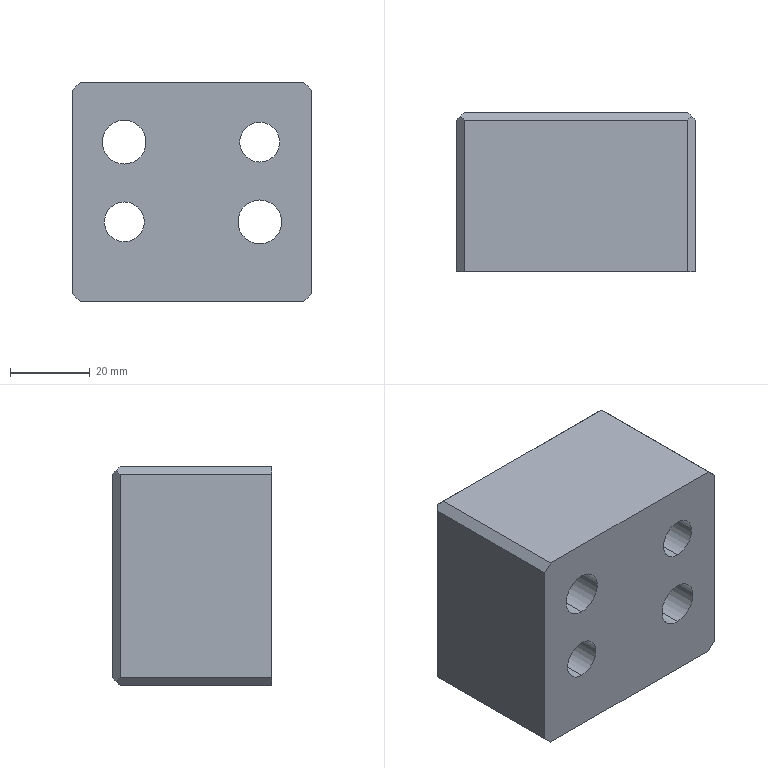Part | Creo | 1 solid | 28 faces | box 60 x 40 x 55 mm | volume 114572 mm3 | plane 16 | cylinder 12 | commonest cylinder face diameters 10 x4 11 x4 16.8 x4
STEP:
#1=CARTESIAN_POINT('',(-185.,390.,-37.));
#2=VERTEX_POINT('',#1);
#3=CARTESIAN_POINT('',(-241.,390.,-37.));
#4=VERTEX_POINT('',#3);
#5=CARTESIAN_POINT('',(-185.,390.,-37.));
#6=DIRECTION('',(-1.,0.,0.));
#7=VECTOR('',#6,56.);
#8=LINE('',#5,#7);
#9=EDGE_CURVE('',#2,#4,#8,.T.);
#10=ORIENTED_EDGE('',*,*,#9,.T.);
#11=CARTESIAN_POINT('',(-241.,390.,-88.));
#12=VERTEX_POINT('',#11);
#13=CARTESIAN_POINT('',(-241.,390.,-37.));
#14=DIRECTION('',(0.,0.,-1.));
#15=VECTOR('',#14,51.);
#16=LINE('',#13,#15);
#17=EDGE_CURVE('',#4,#12,#16,.T.);
#18=ORIENTED_EDGE('',*,*,#17,.T.);
#19=CARTESIAN_POINT('',(-185.,390.,-88.));
#20=VERTEX_POINT('',#19);
#21=CARTESIAN_POINT('',(-241.,390.,-88.));
#22=DIRECTION('',(1.,0.,0.));
#23=VECTOR('',#22,56.);
#24=LINE('',#21,#23);
#25=EDGE_CURVE('',#12,#20,#24,.T.);
#26=ORIENTED_EDGE('',*,*,#25,.T.);
#27=CARTESIAN_POINT('',(-185.,390.,-88.));
#28=DIRECTION('',(0.,0.,1.));
#29=VECTOR('',#28,51.);
#30=LINE('',#27,#29);
#31=EDGE_CURVE('',#20,#2,#30,.T.);
#32=ORIENTED_EDGE('',*,*,#31,.T.);
#33=EDGE_LOOP('',(#10,#18,#26,#32));
#34=FACE_OUTER_BOUND('',#33,.F.);
#35=CARTESIAN_POINT('',(-204.4,390.,-70.));
#36=VERTEX_POINT('',#35);
#37=CARTESIAN_POINT('',(-196.,390.,-78.4));
#38=VERTEX_POINT('',#37);
#39=CARTESIAN_POINT('',(-196.,390.,-70.));
#40=DIRECTION('',(0.,-1.,0.));
#41=DIRECTION('',(-1.,0.,0.));
#42=AXIS2_PLACEMENT_3D('',#39,#40,#41);
#43=CIRCLE('',#42,8.4);
#44=EDGE_CURVE('',#36,#38,#43,.T.);
#45=ORIENTED_EDGE('',*,*,#44,.F.);
#46=CARTESIAN_POINT('',(-196.,390.,-61.6));
#47=VERTEX_POINT('',#46);
#48=CARTESIAN_POINT('',(-196.,390.,-70.));
#49=DIRECTION('',(0.,-1.,0.));
#50=DIRECTION('',(0.,0.,1.));
#51=AXIS2_PLACEMENT_3D('',#48,#49,#50);
#52=CIRCLE('',#51,8.4);
#53=EDGE_CURVE('',#47,#36,#52,.T.);
#54=ORIENTED_EDGE('',*,*,#53,.F.);
#55=CARTESIAN_POINT('',(-196.,390.,-70.));
#56=DIRECTION('',(0.,-1.,0.));
#57=DIRECTION('',(0.,0.,-1.));
#58=AXIS2_PLACEMENT_3D('',#55,#56,#57);
#59=CIRCLE('',#58,8.4);
#60=EDGE_CURVE('',#38,#47,#59,.T.);
#61=ORIENTED_EDGE('',*,*,#60,.F.);
#62=EDGE_LOOP('',(#45,#54,#61));
#63=FACE_BOUND('',#62,.F.);
#64=CARTESIAN_POINT('',(-238.4,390.,-50.));
#65=VERTEX_POINT('',#64);
#66=CARTESIAN_POINT('',(-230.,390.,-58.4));
#67=VERTEX_POINT('',#66);
#68=CARTESIAN_POINT('',(-230.,390.,-50.));
#69=DIRECTION('',(0.,-1.,0.));
#70=DIRECTION('',(-1.,0.,0.));
#71=AXIS2_PLACEMENT_3D('',#68,#69,#70);
#72=CIRCLE('',#71,8.4);
#73=EDGE_CURVE('',#65,#67,#72,.T.);
#74=ORIENTED_EDGE('',*,*,#73,.F.);
#75=CARTESIAN_POINT('',(-230.,390.,-41.6));
#76=VERTEX_POINT('',#75);
#77=CARTESIAN_POINT('',(-230.,390.,-50.));
#78=DIRECTION('',(0.,-1.,0.));
#79=DIRECTION('',(0.,0.,1.));
#80=AXIS2_PLACEMENT_3D('',#77,#78,#79);
#81=CIRCLE('',#80,8.4);
#82=EDGE_CURVE('',#76,#65,#81,.T.);
#83=ORIENTED_EDGE('',*,*,#82,.F.);
#84=CARTESIAN_POINT('',(-230.,390.,-50.));
#85=DIRECTION('',(0.,-1.,0.));
#86=DIRECTION('',(0.,0.,-1.));
#87=AXIS2_PLACEMENT_3D('',#84,#85,#86);
#88=CIRCLE('',#87,8.4);
#89=EDGE_CURVE('',#67,#76,#88,.T.);
#90=ORIENTED_EDGE('',*,*,#89,.F.);
#91=EDGE_LOOP('',(#74,#83,#90));
#92=FACE_BOUND('',#91,.F.);
#93=CARTESIAN_POINT('',(-230.,390.,-75.));
#94=VERTEX_POINT('',#93);
#95=CARTESIAN_POINT('',(-230.,390.,-65.));
#96=VERTEX_POINT('',#95);
#97=CARTESIAN_POINT('',(-230.,390.,-70.));
#98=DIRECTION('',(0.,-1.,0.));
#99=DIRECTION('',(0.,0.,-1.));
#100=AXIS2_PLACEMENT_3D('',#97,#98,#99);
#101=CIRCLE('',#100,5.);
#102=EDGE_CURVE('',#94,#96,#101,.T.);
#103=ORIENTED_EDGE('',*,*,#102,.F.);
#104=CARTESIAN_POINT('',(-230.,390.,-70.));
#105=DIRECTION('',(0.,-1.,0.));
#106=DIRECTION('',(0.,0.,1.));
#107=AXIS2_PLACEMENT_3D('',#104,#105,#106);
#108=CIRCLE('',#107,5.);
#109=EDGE_CURVE('',#96,#94,#108,.T.);
#110=ORIENTED_EDGE('',*,*,#109,.F.);
#111=EDGE_LOOP('',(#103,#110));
#112=FACE_BOUND('',#111,.F.);
#113=CARTESIAN_POINT('',(-196.,390.,-55.));
#114=VERTEX_POINT('',#113);
#115=CARTESIAN_POINT('',(-196.,390.,-45.));
#116=VERTEX_POINT('',#115);
#117=CARTESIAN_POINT('',(-196.,390.,-50.));
#118=DIRECTION('',(0.,-1.,0.));
#119=DIRECTION('',(0.,0.,-1.));
#120=AXIS2_PLACEMENT_3D('',#117,#118,#119);
#121=CIRCLE('',#120,5.);
#122=EDGE_CURVE('',#114,#116,#121,.T.);
#123=ORIENTED_EDGE('',*,*,#122,.F.);
#124=CARTESIAN_POINT('',(-196.,390.,-50.));
#125=DIRECTION('',(0.,-1.,0.));
#126=DIRECTION('',(0.,0.,1.));
#127=AXIS2_PLACEMENT_3D('',#124,#125,#126);
#128=CIRCLE('',#127,5.);
#129=EDGE_CURVE('',#116,#114,#128,.T.);
#130=ORIENTED_EDGE('',*,*,#129,.F.);
#131=EDGE_LOOP('',(#123,#130));
#132=FACE_BOUND('',#131,.F.);
#133=CARTESIAN_POINT('',(322.5,390.,70.));
#134=DIRECTION('',(0.,1.,0.));
#135=DIRECTION('',(0.,0.,-1.));
#136=AXIS2_PLACEMENT_3D('',#133,#134,#135);
#137=PLANE('',#136);
#138=ADVANCED_FACE('',(#34,#63,#92,#112,#132),#137,.T.);
#139=ORIENTED_EDGE('',*,*,#82,.T.);
#140=ORIENTED_EDGE('',*,*,#73,.T.);
#141=CARTESIAN_POINT('',(-230.,379.,-58.4));
#142=VERTEX_POINT('',#141);
#143=CARTESIAN_POINT('',(-230.,379.,-58.4));
#144=DIRECTION('',(0.,1.,0.));
#145=VECTOR('',#144,11.);
#146=LINE('',#143,#145);
#147=EDGE_CURVE('',#142,#67,#146,.T.);
#148=ORIENTED_EDGE('',*,*,#147,.F.);
#149=CARTESIAN_POINT('',(-238.4,379.,-50.));
#150=VERTEX_POINT('',#149);
#151=CARTESIAN_POINT('',(-230.,379.,-50.));
#152=DIRECTION('',(0.,1.,0.));
#153=DIRECTION('',(0.,0.,-1.));
#154=AXIS2_PLACEMENT_3D('',#151,#152,#153);
#155=CIRCLE('',#154,8.4);
#156=EDGE_CURVE('',#142,#150,#155,.T.);
#157=ORIENTED_EDGE('',*,*,#156,.T.);
#158=CARTESIAN_POINT('',(-230.,379.,-41.6));
#159=VERTEX_POINT('',#158);
#160=CARTESIAN_POINT('',(-230.,379.,-50.));
#161=DIRECTION('',(0.,1.,0.));
#162=DIRECTION('',(-1.,0.,0.));
#163=AXIS2_PLACEMENT_3D('',#160,#161,#162);
#164=CIRCLE('',#163,8.4);
#165=EDGE_CURVE('',#150,#159,#164,.T.);
#166=ORIENTED_EDGE('',*,*,#165,.T.);
#167=CARTESIAN_POINT('',(-230.,379.,-41.6));
#168=DIRECTION('',(0.,1.,0.));
#169=VECTOR('',#168,11.);
#170=LINE('',#167,#169);
#171=EDGE_CURVE('',#159,#76,#170,.T.);
#172=ORIENTED_EDGE('',*,*,#171,.T.);
#173=EDGE_LOOP('',(#139,#140,#148,#157,#166,#172));
#174=FACE_OUTER_BOUND('',#173,.F.);
#175=CARTESIAN_POINT('',(-230.,379.,-50.));
#176=DIRECTION('',(0.,1.,0.));
#177=DIRECTION('',(0.,0.,-1.));
#178=AXIS2_PLACEMENT_3D('',#175,#176,#177);
#179=CYLINDRICAL_SURFACE('',#178,8.4);
#180=ADVANCED_FACE('',(#174),#179,.F.);
#181=ORIENTED_EDGE('',*,*,#89,.T.);
#182=ORIENTED_EDGE('',*,*,#171,.F.);
#183=CARTESIAN_POINT('',(-221.6,379.,-50.));
#184=VERTEX_POINT('',#183);
#185=CARTESIAN_POINT('',(-230.,379.,-50.));
#186=DIRECTION('',(0.,1.,0.));
#187=DIRECTION('',(0.,0.,1.));
#188=AXIS2_PLACEMENT_3D('',#185,#186,#187);
#189=CIRCLE('',#188,8.4);
#190=EDGE_CURVE('',#159,#184,#189,.T.);
#191=ORIENTED_EDGE('',*,*,#190,.T.);
#192=CARTESIAN_POINT('',(-230.,379.,-50.));
#193=DIRECTION('',(0.,1.,0.));
#194=DIRECTION('',(1.,0.,0.));
#195=AXIS2_PLACEMENT_3D('',#192,#193,#194);
#196=CIRCLE('',#195,8.4);
#197=EDGE_CURVE('',#184,#142,#196,.T.);
#198=ORIENTED_EDGE('',*,*,#197,.T.);
#199=ORIENTED_EDGE('',*,*,#147,.T.);
#200=EDGE_LOOP('',(#181,#182,#191,#198,#199));
#201=FACE_OUTER_BOUND('',#200,.F.);
#202=CARTESIAN_POINT('',(-230.,379.,-50.));
#203=DIRECTION('',(0.,1.,0.));
#204=DIRECTION('',(0.,0.,-1.));
#205=AXIS2_PLACEMENT_3D('',#202,#203,#204);
#206=CYLINDRICAL_SURFACE('',#205,8.4);
#207=ADVANCED_FACE('',(#201),#206,.F.);
#208=ORIENTED_EDGE('',*,*,#165,.F.);
#209=ORIENTED_EDGE('',*,*,#156,.F.);
#210=ORIENTED_EDGE('',*,*,#197,.F.);
#211=ORIENTED_EDGE('',*,*,#190,.F.);
#212=EDGE_LOOP('',(#208,#209,#210,#211));
#213=FACE_OUTER_BOUND('',#212,.F.);
#214=CARTESIAN_POINT('',(-230.,379.,-55.5));
#215=VERTEX_POINT('',#214);
#216=CARTESIAN_POINT('',(-230.,379.,-44.5));
#217=VERTEX_POINT('',#216);
#218=CARTESIAN_POINT('',(-230.,379.,-50.));
#219=DIRECTION('',(0.,-1.,0.));
#220=DIRECTION('',(0.,0.,-1.));
#221=AXIS2_PLACEMENT_3D('',#218,#219,#220);
#222=CIRCLE('',#221,5.5);
#223=EDGE_CURVE('',#215,#217,#222,.T.);
#224=ORIENTED_EDGE('',*,*,#223,.F.);
#225=CARTESIAN_POINT('',(-230.,379.,-50.));
#226=DIRECTION('',(0.,-1.,0.));
#227=DIRECTION('',(0.,0.,1.));
#228=AXIS2_PLACEMENT_3D('',#225,#226,#227);
#229=CIRCLE('',#228,5.5);
#230=EDGE_CURVE('',#217,#215,#229,.T.);
#231=ORIENTED_EDGE('',*,*,#230,.F.);
#232=EDGE_LOOP('',(#224,#231));
#233=FACE_BOUND('',#232,.F.);
#234=CARTESIAN_POINT('',(22.5,379.,64.5));
#235=DIRECTION('',(0.,1.,0.));
#236=DIRECTION('',(0.,0.,-1.));
#237=AXIS2_PLACEMENT_3D('',#234,#235,#236);
#238=PLANE('',#237);
#239=ADVANCED_FACE('',(#213,#233),#238,.T.);
#240=CARTESIAN_POINT('',(-230.,350.,-44.5));
#241=VERTEX_POINT('',#240);
#242=CARTESIAN_POINT('',(-230.,350.,-55.5));
#243=VERTEX_POINT('',#242);
#244=CARTESIAN_POINT('',(-230.,350.,-50.));
#245=DIRECTION('',(0.,1.,0.));
#246=DIRECTION('',(0.,0.,1.));
#247=AXIS2_PLACEMENT_3D('',#244,#245,#246);
#248=CIRCLE('',#247,5.5);
#249=EDGE_CURVE('',#241,#243,#248,.T.);
#250=ORIENTED_EDGE('',*,*,#249,.T.);
#251=CARTESIAN_POINT('',(-230.,350.,-55.5));
#252=DIRECTION('',(0.,1.,0.));
#253=VECTOR('',#252,29.);
#254=LINE('',#251,#253);
#255=EDGE_CURVE('',#243,#215,#254,.T.);
#256=ORIENTED_EDGE('',*,*,#255,.T.);
#257=ORIENTED_EDGE('',*,*,#223,.T.);
#258=CARTESIAN_POINT('',(-230.,350.,-44.5));
#259=DIRECTION('',(0.,1.,0.));
#260=VECTOR('',#259,29.);
#261=LINE('',#258,#260);
#262=EDGE_CURVE('',#241,#217,#261,.T.);
#263=ORIENTED_EDGE('',*,*,#262,.F.);
#264=EDGE_LOOP('',(#250,#256,#257,#263));
#265=FACE_OUTER_BOUND('',#264,.F.);
#266=CARTESIAN_POINT('',(-230.,390.,-50.));
#267=DIRECTION('',(0.,1.,0.));
#268=DIRECTION('',(0.,0.,-1.));
#269=AXIS2_PLACEMENT_3D('',#266,#267,#268);
#270=CYLINDRICAL_SURFACE('',#269,5.5);
#271=ADVANCED_FACE('',(#265),#270,.F.);
#272=CARTESIAN_POINT('',(-183.,350.,-88.));
#273=VERTEX_POINT('',#272);
#274=CARTESIAN_POINT('',(-183.,350.,-37.));
#275=VERTEX_POINT('',#274);
#276=CARTESIAN_POINT('',(-183.,350.,-88.));
#277=DIRECTION('',(0.,0.,1.));
#278=VECTOR('',#277,51.);
#279=LINE('',#276,#278);
#280=EDGE_CURVE('',#273,#275,#279,.T.);
#281=ORIENTED_EDGE('',*,*,#280,.F.);
#282=CARTESIAN_POINT('',(-185.,350.,-90.));
#283=VERTEX_POINT('',#282);
#284=CARTESIAN_POINT('',(-185.,350.,-90.));
#285=DIRECTION('',(0.7071,0.,0.7071));
#286=VECTOR('',#285,2.828);
#287=LINE('',#284,#286);
#288=EDGE_CURVE('',#283,#273,#287,.T.);
#289=ORIENTED_EDGE('',*,*,#288,.F.);
#290=CARTESIAN_POINT('',(-241.,350.,-90.));
#291=VERTEX_POINT('',#290);
#292=CARTESIAN_POINT('',(-241.,350.,-90.));
#293=DIRECTION('',(1.,0.,0.));
#294=VECTOR('',#293,56.);
#295=LINE('',#292,#294);
#296=EDGE_CURVE('',#291,#283,#295,.T.);
#297=ORIENTED_EDGE('',*,*,#296,.F.);
#298=CARTESIAN_POINT('',(-243.,350.,-88.));
#299=VERTEX_POINT('',#298);
#300=CARTESIAN_POINT('',(-243.,350.,-88.));
#301=DIRECTION('',(0.7071,0.,-0.7071));
#302=VECTOR('',#301,2.828);
#303=LINE('',#300,#302);
#304=EDGE_CURVE('',#299,#291,#303,.T.);
#305=ORIENTED_EDGE('',*,*,#304,.F.);
#306=CARTESIAN_POINT('',(-243.,350.,-37.));
#307=VERTEX_POINT('',#306);
#308=CARTESIAN_POINT('',(-243.,350.,-37.));
#309=DIRECTION('',(0.,0.,-1.));
#310=VECTOR('',#309,51.);
#311=LINE('',#308,#310);
#312=EDGE_CURVE('',#307,#299,#311,.T.);
#313=ORIENTED_EDGE('',*,*,#312,.F.);
#314=CARTESIAN_POINT('',(-241.,350.,-35.));
#315=VERTEX_POINT('',#314);
#316=CARTESIAN_POINT('',(-241.,350.,-35.));
#317=DIRECTION('',(-0.7071,0.,-0.7071));
#318=VECTOR('',#317,2.828);
#319=LINE('',#316,#318);
#320=EDGE_CURVE('',#315,#307,#319,.T.);
#321=ORIENTED_EDGE('',*,*,#320,.F.);
#322=CARTESIAN_POINT('',(-185.,350.,-35.));
#323=VERTEX_POINT('',#322);
#324=CARTESIAN_POINT('',(-185.,350.,-35.));
#325=DIRECTION('',(-1.,0.,0.));
#326=VECTOR('',#325,56.);
#327=LINE('',#324,#326);
#328=EDGE_CURVE('',#323,#315,#327,.T.);
#329=ORIENTED_EDGE('',*,*,#328,.F.);
#330=CARTESIAN_POINT('',(-183.,350.,-37.));
#331=DIRECTION('',(-0.7071,0.,0.7071));
#332=VECTOR('',#331,2.828);
#333=LINE('',#330,#332);
#334=EDGE_CURVE('',#275,#323,#333,.T.);
#335=ORIENTED_EDGE('',*,*,#334,.F.);
#336=EDGE_LOOP('',(#281,#289,#297,#305,#313,#321,#329,#335));
#337=FACE_OUTER_BOUND('',#336,.F.);
#338=CARTESIAN_POINT('',(-196.,350.,-75.5));
#339=VERTEX_POINT('',#338);
#340=CARTESIAN_POINT('',(-196.,350.,-64.5));
#341=VERTEX_POINT('',#340);
#342=CARTESIAN_POINT('',(-196.,350.,-70.));
#343=DIRECTION('',(0.,1.,0.));
#344=DIRECTION('',(0.,0.,-1.));
#345=AXIS2_PLACEMENT_3D('',#342,#343,#344);
#346=CIRCLE('',#345,5.5);
#347=EDGE_CURVE('',#339,#341,#346,.T.);
#348=ORIENTED_EDGE('',*,*,#347,.F.);
#349=CARTESIAN_POINT('',(-196.,350.,-70.));
#350=DIRECTION('',(0.,1.,0.));
#351=DIRECTION('',(0.,0.,1.));
#352=AXIS2_PLACEMENT_3D('',#349,#350,#351);
#353=CIRCLE('',#352,5.5);
#354=EDGE_CURVE('',#341,#339,#353,.T.);
#355=ORIENTED_EDGE('',*,*,#354,.F.);
#356=EDGE_LOOP('',(#348,#355));
#357=FACE_BOUND('',#356,.F.);
#358=CARTESIAN_POINT('',(-230.,350.,-50.));
#359=DIRECTION('',(0.,1.,0.));
#360=DIRECTION('',(0.,0.,-1.));
#361=AXIS2_PLACEMENT_3D('',#358,#359,#360);
#362=CIRCLE('',#361,5.5);
#363=EDGE_CURVE('',#243,#241,#362,.T.);
#364=ORIENTED_EDGE('',*,*,#363,.F.);
#365=ORIENTED_EDGE('',*,*,#249,.F.);
#366=EDGE_LOOP('',(#364,#365));
#367=FACE_BOUND('',#366,.F.);
#368=CARTESIAN_POINT('',(-230.,350.,-75.));
#369=VERTEX_POINT('',#368);
#370=CARTESIAN_POINT('',(-230.,350.,-65.));
#371=VERTEX_POINT('',#370);
#372=CARTESIAN_POINT('',(-230.,350.,-70.));
#373=DIRECTION('',(0.,1.,0.));
#374=DIRECTION('',(0.,0.,-1.));
#375=AXIS2_PLACEMENT_3D('',#372,#373,#374);
#376=CIRCLE('',#375,5.);
#377=EDGE_CURVE('',#369,#371,#376,.T.);
#378=ORIENTED_EDGE('',*,*,#377,.F.);
#379=CARTESIAN_POINT('',(-230.,350.,-70.));
#380=DIRECTION('',(0.,1.,0.));
#381=DIRECTION('',(0.,0.,1.));
#382=AXIS2_PLACEMENT_3D('',#379,#380,#381);
#383=CIRCLE('',#382,5.);
#384=EDGE_CURVE('',#371,#369,#383,.T.);
#385=ORIENTED_EDGE('',*,*,#384,.F.);
#386=EDGE_LOOP('',(#378,#385));
#387=FACE_BOUND('',#386,.F.);
#388=CARTESIAN_POINT('',(-196.,350.,-55.));
#389=VERTEX_POINT('',#388);
#390=CARTESIAN_POINT('',(-196.,350.,-45.));
#391=VERTEX_POINT('',#390);
#392=CARTESIAN_POINT('',(-196.,350.,-50.));
#393=DIRECTION('',(0.,1.,0.));
#394=DIRECTION('',(0.,0.,-1.));
#395=AXIS2_PLACEMENT_3D('',#392,#393,#394);
#396=CIRCLE('',#395,5.);
#397=EDGE_CURVE('',#389,#391,#396,.T.);
#398=ORIENTED_EDGE('',*,*,#397,.F.);
#399=CARTESIAN_POINT('',(-196.,350.,-50.));
#400=DIRECTION('',(0.,1.,0.));
#401=DIRECTION('',(0.,0.,1.));
#402=AXIS2_PLACEMENT_3D('',#399,#400,#401);
#403=CIRCLE('',#402,5.);
#404=EDGE_CURVE('',#391,#389,#403,.T.);
#405=ORIENTED_EDGE('',*,*,#404,.F.);
#406=EDGE_LOOP('',(#398,#405));
#407=FACE_BOUND('',#406,.F.);
#408=CARTESIAN_POINT('',(322.5,350.,70.));
#409=DIRECTION('',(0.,1.,0.));
#410=DIRECTION('',(0.,0.,-1.));
#411=AXIS2_PLACEMENT_3D('',#408,#409,#410);
#412=PLANE('',#411);
#413=ADVANCED_FACE('',(#337,#357,#367,#387,#407),#412,.F.);
#414=CARTESIAN_POINT('',(-183.,388.,-88.));
#415=VERTEX_POINT('',#414);
#416=CARTESIAN_POINT('',(-183.,388.,-37.));
#417=VERTEX_POINT('',#416);
#418=CARTESIAN_POINT('',(-183.,388.,-88.));
#419=DIRECTION('',(0.,0.,1.));
#420=VECTOR('',#419,51.);
#421=LINE('',#418,#420);
#422=EDGE_CURVE('',#415,#417,#421,.T.);
#423=ORIENTED_EDGE('',*,*,#422,.F.);
#424=CARTESIAN_POINT('',(-183.,350.,-88.));
#425=DIRECTION('',(0.,1.,0.));
#426=VECTOR('',#425,38.);
#427=LINE('',#424,#426);
#428=EDGE_CURVE('',#273,#415,#427,.T.);
#429=ORIENTED_EDGE('',*,*,#428,.F.);
#430=ORIENTED_EDGE('',*,*,#280,.T.);
#431=CARTESIAN_POINT('',(-183.,350.,-37.));
#432=DIRECTION('',(0.,1.,0.));
#433=VECTOR('',#432,38.);
#434=LINE('',#431,#433);
#435=EDGE_CURVE('',#275,#417,#434,.T.);
#436=ORIENTED_EDGE('',*,*,#435,.T.);
#437=EDGE_LOOP('',(#423,#429,#430,#436));
#438=FACE_OUTER_BOUND('',#437,.F.);
#439=CARTESIAN_POINT('',(-183.,350.,-30.));
#440=DIRECTION('',(1.,0.,0.));
#441=DIRECTION('',(0.,0.,1.));
#442=AXIS2_PLACEMENT_3D('',#439,#440,#441);
#443=PLANE('',#442);
#444=ADVANCED_FACE('',(#438),#443,.T.);
#445=CARTESIAN_POINT('',(-184.,389.,-36.));
#446=VERTEX_POINT('',#445);
#447=CARTESIAN_POINT('',(-184.,389.,-36.));
#448=DIRECTION('',(-0.5774,0.5774,-0.5774));
#449=VECTOR('',#448,1.732);
#450=LINE('',#447,#449);
#451=EDGE_CURVE('',#446,#2,#450,.T.);
#452=ORIENTED_EDGE('',*,*,#451,.T.);
#453=ORIENTED_EDGE('',*,*,#31,.F.);
#454=CARTESIAN_POINT('',(-184.,389.,-89.));
#455=VERTEX_POINT('',#454);
#456=CARTESIAN_POINT('',(-185.,390.,-88.));
#457=DIRECTION('',(0.5774,-0.5774,-0.5774));
#458=VECTOR('',#457,1.732);
#459=LINE('',#456,#458);
#460=EDGE_CURVE('',#20,#455,#459,.T.);
#461=ORIENTED_EDGE('',*,*,#460,.T.);
#462=CARTESIAN_POINT('',(-184.,389.,-89.));
#463=DIRECTION('',(0.5774,-0.5774,0.5774));
#464=VECTOR('',#463,1.732);
#465=LINE('',#462,#464);
#466=EDGE_CURVE('',#455,#415,#465,.T.);
#467=ORIENTED_EDGE('',*,*,#466,.T.);
#468=ORIENTED_EDGE('',*,*,#422,.T.);
#469=CARTESIAN_POINT('',(-184.,389.,-36.));
#470=DIRECTION('',(0.5774,-0.5774,-0.5774));
#471=VECTOR('',#470,1.732);
#472=LINE('',#469,#471);
#473=EDGE_CURVE('',#446,#417,#472,.T.);
#474=ORIENTED_EDGE('',*,*,#473,.F.);
#475=EDGE_LOOP('',(#452,#453,#461,#467,#468,#474));
#476=FACE_OUTER_BOUND('',#475,.F.);
#477=CARTESIAN_POINT('',(-184.,389.,-60.));
#478=DIRECTION('',(0.7071,0.7071,0.));
#479=DIRECTION('',(-0.7071,0.7071,0.));
#480=AXIS2_PLACEMENT_3D('',#477,#478,#479);
#481=PLANE('',#480);
#482=ADVANCED_FACE('',(#476),#481,.T.);
#483=CARTESIAN_POINT('',(-185.,388.,-35.));
#484=VERTEX_POINT('',#483);
#485=CARTESIAN_POINT('',(-185.,388.,-35.));
#486=DIRECTION('',(0.5774,0.5774,-0.5774));
#487=VECTOR('',#486,1.732);
#488=LINE('',#485,#487);
#489=EDGE_CURVE('',#484,#446,#488,.T.);
#490=ORIENTED_EDGE('',*,*,#489,.F.);
#491=CARTESIAN_POINT('',(-241.,388.,-35.));
#492=VERTEX_POINT('',#491);
#493=CARTESIAN_POINT('',(-185.,388.,-35.));
#494=DIRECTION('',(-1.,0.,0.));
#495=VECTOR('',#494,56.);
#496=LINE('',#493,#495);
#497=EDGE_CURVE('',#484,#492,#496,.T.);
#498=ORIENTED_EDGE('',*,*,#497,.T.);
#499=CARTESIAN_POINT('',(-242.,389.,-36.));
#500=VERTEX_POINT('',#499);
#501=CARTESIAN_POINT('',(-242.,389.,-36.));
#502=DIRECTION('',(0.5774,-0.5774,0.5774));
#503=VECTOR('',#502,1.732);
#504=LINE('',#501,#503);
#505=EDGE_CURVE('',#500,#492,#504,.T.);
#506=ORIENTED_EDGE('',*,*,#505,.F.);
#507=CARTESIAN_POINT('',(-242.,389.,-36.));
#508=DIRECTION('',(0.5774,0.5774,-0.5774));
#509=VECTOR('',#508,1.732);
#510=LINE('',#507,#509);
#511=EDGE_CURVE('',#500,#4,#510,.T.);
#512=ORIENTED_EDGE('',*,*,#511,.T.);
#513=ORIENTED_EDGE('',*,*,#9,.F.);
#514=ORIENTED_EDGE('',*,*,#451,.F.);
#515=EDGE_LOOP('',(#490,#498,#506,#512,#513,#514));
#516=FACE_OUTER_BOUND('',#515,.F.);
#517=CARTESIAN_POINT('',(-213.,389.,-36.));
#518=DIRECTION('',(0.,0.7071,0.7071));
#519=DIRECTION('',(0.,0.7071,-0.7071));
#520=AXIS2_PLACEMENT_3D('',#517,#518,#519);
#521=PLANE('',#520);
#522=ADVANCED_FACE('',(#516),#521,.T.);
#523=ORIENTED_EDGE('',*,*,#435,.F.);
#524=ORIENTED_EDGE('',*,*,#334,.T.);
#525=CARTESIAN_POINT('',(-185.,350.,-35.));
#526=DIRECTION('',(0.,1.,0.));
#527=VECTOR('',#526,38.);
#528=LINE('',#525,#527);
#529=EDGE_CURVE('',#323,#484,#528,.T.);
#530=ORIENTED_EDGE('',*,*,#529,.T.);
#531=ORIENTED_EDGE('',*,*,#489,.T.);
#532=ORIENTED_EDGE('',*,*,#473,.T.);
#533=EDGE_LOOP('',(#523,#524,#530,#531,#532));
#534=FACE_OUTER_BOUND('',#533,.F.);
#535=CARTESIAN_POINT('',(-184.,370.,-36.));
#536=DIRECTION('',(0.7071,0.,0.7071));
#537=DIRECTION('',(-0.7071,0.,0.7071));
#538=AXIS2_PLACEMENT_3D('',#535,#536,#537);
#539=PLANE('',#538);
#540=ADVANCED_FACE('',(#534),#539,.T.);
#541=ORIENTED_EDGE('',*,*,#328,.T.);
#542=CARTESIAN_POINT('',(-241.,350.,-35.));
#543=DIRECTION('',(0.,1.,0.));
#544=VECTOR('',#543,38.);
#545=LINE('',#542,#544);
#546=EDGE_CURVE('',#315,#492,#545,.T.);
#547=ORIENTED_EDGE('',*,*,#546,.T.);
#548=ORIENTED_EDGE('',*,*,#497,.F.);
#549=ORIENTED_EDGE('',*,*,#529,.F.);
#550=EDGE_LOOP('',(#541,#547,#548,#549));
#551=FACE_OUTER_BOUND('',#550,.F.);
#552=CARTESIAN_POINT('',(-243.,350.,-35.));
#553=DIRECTION('',(0.,0.,1.));
#554=DIRECTION('',(-1.,0.,0.));
#555=AXIS2_PLACEMENT_3D('',#552,#553,#554);
#556=PLANE('',#555);
#557=ADVANCED_FACE('',(#551),#556,.T.);
#558=ORIENTED_EDGE('',*,*,#546,.F.);
#559=ORIENTED_EDGE('',*,*,#320,.T.);
#560=CARTESIAN_POINT('',(-243.,388.,-37.));
#561=VERTEX_POINT('',#560);
#562=CARTESIAN_POINT('',(-243.,350.,-37.));
#563=DIRECTION('',(0.,1.,0.));
#564=VECTOR('',#563,38.);
#565=LINE('',#562,#564);
#566=EDGE_CURVE('',#307,#561,#565,.T.);
#567=ORIENTED_EDGE('',*,*,#566,.T.);
#568=CARTESIAN_POINT('',(-243.,388.,-37.));
#569=DIRECTION('',(0.5774,0.5774,0.5774));
#570=VECTOR('',#569,1.732);
#571=LINE('',#568,#570);
#572=EDGE_CURVE('',#561,#500,#571,.T.);
#573=ORIENTED_EDGE('',*,*,#572,.T.);
#574=ORIENTED_EDGE('',*,*,#505,.T.);
#575=EDGE_LOOP('',(#558,#559,#567,#573,#574));
#576=FACE_OUTER_BOUND('',#575,.F.);
#577=CARTESIAN_POINT('',(-242.,370.,-36.));
#578=DIRECTION('',(-0.7071,0.,0.7071));
#579=DIRECTION('',(-0.7071,0.,-0.7071));
#580=AXIS2_PLACEMENT_3D('',#577,#578,#579);
#581=PLANE('',#580);
#582=ADVANCED_FACE('',(#576),#581,.T.);
#583=ORIENTED_EDGE('',*,*,#312,.T.);
#584=CARTESIAN_POINT('',(-243.,388.,-88.));
#585=VERTEX_POINT('',#584);
#586=CARTESIAN_POINT('',(-243.,350.,-88.));
#587=DIRECTION('',(0.,1.,0.));
#588=VECTOR('',#587,38.);
#589=LINE('',#586,#588);
#590=EDGE_CURVE('',#299,#585,#589,.T.);
#591=ORIENTED_EDGE('',*,*,#590,.T.);
#592=CARTESIAN_POINT('',(-243.,388.,-37.));
#593=DIRECTION('',(0.,0.,-1.));
#594=VECTOR('',#593,51.);
#595=LINE('',#592,#594);
#596=EDGE_CURVE('',#561,#585,#595,.T.);
#597=ORIENTED_EDGE('',*,*,#596,.F.);
#598=ORIENTED_EDGE('',*,*,#566,.F.);
#599=EDGE_LOOP('',(#583,#591,#597,#598));
#600=FACE_OUTER_BOUND('',#599,.F.);
#601=CARTESIAN_POINT('',(-243.,350.,-90.));
#602=DIRECTION('',(-1.,0.,0.));
#603=DIRECTION('',(0.,0.,-1.));
#604=AXIS2_PLACEMENT_3D('',#601,#602,#603);
#605=PLANE('',#604);
#606=ADVANCED_FACE('',(#600),#605,.T.);
#607=ORIENTED_EDGE('',*,*,#590,.F.);
#608=ORIENTED_EDGE('',*,*,#304,.T.);
#609=CARTESIAN_POINT('',(-241.,388.,-90.));
#610=VERTEX_POINT('',#609);
#611=CARTESIAN_POINT('',(-241.,350.,-90.));
#612=DIRECTION('',(0.,1.,0.));
#613=VECTOR('',#612,38.);
#614=LINE('',#611,#613);
#615=EDGE_CURVE('',#291,#610,#614,.T.);
#616=ORIENTED_EDGE('',*,*,#615,.T.);
#617=CARTESIAN_POINT('',(-242.,389.,-89.));
#618=VERTEX_POINT('',#617);
#619=CARTESIAN_POINT('',(-241.,388.,-90.));
#620=DIRECTION('',(-0.5774,0.5774,0.5774));
#621=VECTOR('',#620,1.732);
#622=LINE('',#619,#621);
#623=EDGE_CURVE('',#610,#618,#622,.T.);
#624=ORIENTED_EDGE('',*,*,#623,.T.);
#625=CARTESIAN_POINT('',(-242.,389.,-89.));
#626=DIRECTION('',(-0.5774,-0.5774,0.5774));
#627=VECTOR('',#626,1.732);
#628=LINE('',#625,#627);
#629=EDGE_CURVE('',#618,#585,#628,.T.);
#630=ORIENTED_EDGE('',*,*,#629,.T.);
#631=EDGE_LOOP('',(#607,#608,#616,#624,#630));
#632=FACE_OUTER_BOUND('',#631,.F.);
#633=CARTESIAN_POINT('',(-242.,370.,-89.));
#634=DIRECTION('',(-0.7071,0.,-0.7071));
#635=DIRECTION('',(0.7071,0.,-0.7071));
#636=AXIS2_PLACEMENT_3D('',#633,#634,#635);
#637=PLANE('',#636);
#638=ADVANCED_FACE('',(#632),#637,.T.);
#639=ORIENTED_EDGE('',*,*,#296,.T.);
#640=CARTESIAN_POINT('',(-185.,388.,-90.));
#641=VERTEX_POINT('',#640);
#642=CARTESIAN_POINT('',(-185.,350.,-90.));
#643=DIRECTION('',(0.,1.,0.));
#644=VECTOR('',#643,38.);
#645=LINE('',#642,#644);
#646=EDGE_CURVE('',#283,#641,#645,.T.);
#647=ORIENTED_EDGE('',*,*,#646,.T.);
#648=CARTESIAN_POINT('',(-241.,388.,-90.));
#649=DIRECTION('',(1.,0.,0.));
#650=VECTOR('',#649,56.);
#651=LINE('',#648,#650);
#652=EDGE_CURVE('',#610,#641,#651,.T.);
#653=ORIENTED_EDGE('',*,*,#652,.F.);
#654=ORIENTED_EDGE('',*,*,#615,.F.);
#655=EDGE_LOOP('',(#639,#647,#653,#654));
#656=FACE_OUTER_BOUND('',#655,.F.);
#657=CARTESIAN_POINT('',(-183.,350.,-90.));
#658=DIRECTION('',(0.,0.,-1.));
#659=DIRECTION('',(1.,0.,0.));
#660=AXIS2_PLACEMENT_3D('',#657,#658,#659);
#661=PLANE('',#660);
#662=ADVANCED_FACE('',(#656),#661,.T.);
#663=ORIENTED_EDGE('',*,*,#646,.F.);
#664=ORIENTED_EDGE('',*,*,#288,.T.);
#665=ORIENTED_EDGE('',*,*,#428,.T.);
#666=ORIENTED_EDGE('',*,*,#466,.F.);
#667=CARTESIAN_POINT('',(-184.,389.,-89.));
#668=DIRECTION('',(-0.5774,-0.5774,-0.5774));
#669=VECTOR('',#668,1.732);
#670=LINE('',#667,#669);
#671=EDGE_CURVE('',#455,#641,#670,.T.);
#672=ORIENTED_EDGE('',*,*,#671,.T.);
#673=EDGE_LOOP('',(#663,#664,#665,#666,#672));
#674=FACE_OUTER_BOUND('',#673,.F.);
#675=CARTESIAN_POINT('',(-184.,370.,-89.));
#676=DIRECTION('',(0.7071,0.,-0.7071));
#677=DIRECTION('',(0.7071,0.,0.7071));
#678=AXIS2_PLACEMENT_3D('',#675,#676,#677);
#679=PLANE('',#678);
#680=ADVANCED_FACE('',(#674),#679,.T.);
#681=ORIENTED_EDGE('',*,*,#623,.F.);
#682=ORIENTED_EDGE('',*,*,#652,.T.);
#683=ORIENTED_EDGE('',*,*,#671,.F.);
#684=ORIENTED_EDGE('',*,*,#460,.F.);
#685=ORIENTED_EDGE('',*,*,#25,.F.);
#686=CARTESIAN_POINT('',(-242.,389.,-89.));
#687=DIRECTION('',(0.5774,0.5774,0.5774));
#688=VECTOR('',#687,1.732);
#689=LINE('',#686,#688);
#690=EDGE_CURVE('',#618,#12,#689,.T.);
#691=ORIENTED_EDGE('',*,*,#690,.F.);
#692=EDGE_LOOP('',(#681,#682,#683,#684,#685,#691));
#693=FACE_OUTER_BOUND('',#692,.F.);
#694=CARTESIAN_POINT('',(-213.,389.,-89.));
#695=DIRECTION('',(0.,0.7071,-0.7071));
#696=DIRECTION('',(0.,-0.7071,-0.7071));
#697=AXIS2_PLACEMENT_3D('',#694,#695,#696);
#698=PLANE('',#697);
#699=ADVANCED_FACE('',(#693),#698,.T.);
#700=ORIENTED_EDGE('',*,*,#572,.F.);
#701=ORIENTED_EDGE('',*,*,#596,.T.);
#702=ORIENTED_EDGE('',*,*,#629,.F.);
#703=ORIENTED_EDGE('',*,*,#690,.T.);
#704=ORIENTED_EDGE('',*,*,#17,.F.);
#705=ORIENTED_EDGE('',*,*,#511,.F.);
#706=EDGE_LOOP('',(#700,#701,#702,#703,#704,#705));
#707=FACE_OUTER_BOUND('',#706,.F.);
#708=CARTESIAN_POINT('',(-242.,389.,-60.));
#709=DIRECTION('',(-0.7071,0.7071,0.));
#710=DIRECTION('',(-0.7071,-0.7071,0.));
#711=AXIS2_PLACEMENT_3D('',#708,#709,#710);
#712=PLANE('',#711);
#713=ADVANCED_FACE('',(#707),#712,.T.);
#714=ORIENTED_EDGE('',*,*,#347,.T.);
#715=CARTESIAN_POINT('',(-196.,379.,-64.5));
#716=VERTEX_POINT('',#715);
#717=CARTESIAN_POINT('',(-196.,350.,-64.5));
#718=DIRECTION('',(0.,1.,0.));
#719=VECTOR('',#718,29.);
#720=LINE('',#717,#719);
#721=EDGE_CURVE('',#341,#716,#720,.T.);
#722=ORIENTED_EDGE('',*,*,#721,.T.);
#723=CARTESIAN_POINT('',(-196.,379.,-75.5));
#724=VERTEX_POINT('',#723);
#725=CARTESIAN_POINT('',(-196.,379.,-70.));
#726=DIRECTION('',(0.,-1.,0.));
#727=DIRECTION('',(0.,0.,1.));
#728=AXIS2_PLACEMENT_3D('',#725,#726,#727);
#729=CIRCLE('',#728,5.5);
#730=EDGE_CURVE('',#716,#724,#729,.T.);
#731=ORIENTED_EDGE('',*,*,#730,.T.);
#732=CARTESIAN_POINT('',(-196.,350.,-75.5));
#733=DIRECTION('',(0.,1.,0.));
#734=VECTOR('',#733,29.);
#735=LINE('',#732,#734);
#736=EDGE_CURVE('',#339,#724,#735,.T.);
#737=ORIENTED_EDGE('',*,*,#736,.F.);
#738=EDGE_LOOP('',(#714,#722,#731,#737));
#739=FACE_OUTER_BOUND('',#738,.F.);
#740=CARTESIAN_POINT('',(-196.,390.,-70.));
#741=DIRECTION('',(0.,1.,0.));
#742=DIRECTION('',(0.,0.,-1.));
#743=AXIS2_PLACEMENT_3D('',#740,#741,#742);
#744=CYLINDRICAL_SURFACE('',#743,5.5);
#745=ADVANCED_FACE('',(#739),#744,.F.);
#746=ORIENTED_EDGE('',*,*,#354,.T.);
#747=ORIENTED_EDGE('',*,*,#736,.T.);
#748=CARTESIAN_POINT('',(-196.,379.,-70.));
#749=DIRECTION('',(0.,-1.,0.));
#750=DIRECTION('',(0.,0.,-1.));
#751=AXIS2_PLACEMENT_3D('',#748,#749,#750);
#752=CIRCLE('',#751,5.5);
#753=EDGE_CURVE('',#724,#716,#752,.T.);
#754=ORIENTED_EDGE('',*,*,#753,.T.);
#755=ORIENTED_EDGE('',*,*,#721,.F.);
#756=EDGE_LOOP('',(#746,#747,#754,#755));
#757=FACE_OUTER_BOUND('',#756,.F.);
#758=CARTESIAN_POINT('',(-196.,390.,-70.));
#759=DIRECTION('',(0.,1.,0.));
#760=DIRECTION('',(0.,0.,-1.));
#761=AXIS2_PLACEMENT_3D('',#758,#759,#760);
#762=CYLINDRICAL_SURFACE('',#761,5.5);
#763=ADVANCED_FACE('',(#757),#762,.F.);
#764=CARTESIAN_POINT('',(-204.4,379.,-70.));
#765=VERTEX_POINT('',#764);
#766=CARTESIAN_POINT('',(-196.,379.,-61.6));
#767=VERTEX_POINT('',#766);
#768=CARTESIAN_POINT('',(-196.,379.,-70.));
#769=DIRECTION('',(0.,1.,0.));
#770=DIRECTION('',(-1.,0.,0.));
#771=AXIS2_PLACEMENT_3D('',#768,#769,#770);
#772=CIRCLE('',#771,8.4);
#773=EDGE_CURVE('',#765,#767,#772,.T.);
#774=ORIENTED_EDGE('',*,*,#773,.F.);
#775=CARTESIAN_POINT('',(-196.,379.,-78.4));
#776=VERTEX_POINT('',#775);
#777=CARTESIAN_POINT('',(-196.,379.,-70.));
#778=DIRECTION('',(0.,1.,0.));
#779=DIRECTION('',(0.,0.,-1.));
#780=AXIS2_PLACEMENT_3D('',#777,#778,#779);
#781=CIRCLE('',#780,8.4);
#782=EDGE_CURVE('',#776,#765,#781,.T.);
#783=ORIENTED_EDGE('',*,*,#782,.F.);
#784=CARTESIAN_POINT('',(-187.6,379.,-70.));
#785=VERTEX_POINT('',#784);
#786=CARTESIAN_POINT('',(-196.,379.,-70.));
#787=DIRECTION('',(0.,1.,0.));
#788=DIRECTION('',(1.,0.,0.));
#789=AXIS2_PLACEMENT_3D('',#786,#787,#788);
#790=CIRCLE('',#789,8.4);
#791=EDGE_CURVE('',#785,#776,#790,.T.);
#792=ORIENTED_EDGE('',*,*,#791,.F.);
#793=CARTESIAN_POINT('',(-196.,379.,-70.));
#794=DIRECTION('',(0.,1.,0.));
#795=DIRECTION('',(0.,0.,1.));
#796=AXIS2_PLACEMENT_3D('',#793,#794,#795);
#797=CIRCLE('',#796,8.4);
#798=EDGE_CURVE('',#767,#785,#797,.T.);
#799=ORIENTED_EDGE('',*,*,#798,.F.);
#800=EDGE_LOOP('',(#774,#783,#792,#799));
#801=FACE_OUTER_BOUND('',#800,.F.);
#802=ORIENTED_EDGE('',*,*,#753,.F.);
#803=ORIENTED_EDGE('',*,*,#730,.F.);
#804=EDGE_LOOP('',(#802,#803));
#805=FACE_BOUND('',#804,.F.);
#806=CARTESIAN_POINT('',(22.5,379.,74.5));
#807=DIRECTION('',(0.,1.,0.));
#808=DIRECTION('',(0.,0.,-1.));
#809=AXIS2_PLACEMENT_3D('',#806,#807,#808);
#810=PLANE('',#809);
#811=ADVANCED_FACE('',(#801,#805),#810,.T.);
#812=ORIENTED_EDGE('',*,*,#53,.T.);
#813=ORIENTED_EDGE('',*,*,#44,.T.);
#814=CARTESIAN_POINT('',(-196.,379.,-78.4));
#815=DIRECTION('',(0.,1.,0.));
#816=VECTOR('',#815,11.);
#817=LINE('',#814,#816);
#818=EDGE_CURVE('',#776,#38,#817,.T.);
#819=ORIENTED_EDGE('',*,*,#818,.F.);
#820=ORIENTED_EDGE('',*,*,#782,.T.);
#821=ORIENTED_EDGE('',*,*,#773,.T.);
#822=CARTESIAN_POINT('',(-196.,379.,-61.6));
#823=DIRECTION('',(0.,1.,0.));
#824=VECTOR('',#823,11.);
#825=LINE('',#822,#824);
#826=EDGE_CURVE('',#767,#47,#825,.T.);
#827=ORIENTED_EDGE('',*,*,#826,.T.);
#828=EDGE_LOOP('',(#812,#813,#819,#820,#821,#827));
#829=FACE_OUTER_BOUND('',#828,.F.);
#830=CARTESIAN_POINT('',(-196.,379.,-70.));
#831=DIRECTION('',(0.,1.,0.));
#832=DIRECTION('',(0.,0.,-1.));
#833=AXIS2_PLACEMENT_3D('',#830,#831,#832);
#834=CYLINDRICAL_SURFACE('',#833,8.4);
#835=ADVANCED_FACE('',(#829),#834,.F.);
#836=ORIENTED_EDGE('',*,*,#60,.T.);
#837=ORIENTED_EDGE('',*,*,#826,.F.);
#838=ORIENTED_EDGE('',*,*,#798,.T.);
#839=ORIENTED_EDGE('',*,*,#791,.T.);
#840=ORIENTED_EDGE('',*,*,#818,.T.);
#841=EDGE_LOOP('',(#836,#837,#838,#839,#840));
#842=FACE_OUTER_BOUND('',#841,.F.);
#843=CARTESIAN_POINT('',(-196.,379.,-70.));
#844=DIRECTION('',(0.,1.,0.));
#845=DIRECTION('',(0.,0.,-1.));
#846=AXIS2_PLACEMENT_3D('',#843,#844,#845);
#847=CYLINDRICAL_SURFACE('',#846,8.4);
#848=ADVANCED_FACE('',(#842),#847,.F.);
#849=ORIENTED_EDGE('',*,*,#363,.T.);
#850=ORIENTED_EDGE('',*,*,#262,.T.);
#851=ORIENTED_EDGE('',*,*,#230,.T.);
#852=ORIENTED_EDGE('',*,*,#255,.F.);
#853=EDGE_LOOP('',(#849,#850,#851,#852));
#854=FACE_OUTER_BOUND('',#853,.F.);
#855=CARTESIAN_POINT('',(-230.,390.,-50.));
#856=DIRECTION('',(0.,1.,0.));
#857=DIRECTION('',(0.,0.,-1.));
#858=AXIS2_PLACEMENT_3D('',#855,#856,#857);
#859=CYLINDRICAL_SURFACE('',#858,5.5);
#860=ADVANCED_FACE('',(#854),#859,.F.);
#861=ORIENTED_EDGE('',*,*,#377,.T.);
#862=CARTESIAN_POINT('',(-230.,350.,-65.));
#863=DIRECTION('',(0.,1.,0.));
#864=VECTOR('',#863,40.);
#865=LINE('',#862,#864);
#866=EDGE_CURVE('',#371,#96,#865,.T.);
#867=ORIENTED_EDGE('',*,*,#866,.T.);
#868=ORIENTED_EDGE('',*,*,#109,.T.);
#869=CARTESIAN_POINT('',(-230.,350.,-75.));
#870=DIRECTION('',(0.,1.,0.));
#871=VECTOR('',#870,40.);
#872=LINE('',#869,#871);
#873=EDGE_CURVE('',#369,#94,#872,.T.);
#874=ORIENTED_EDGE('',*,*,#873,.F.);
#875=EDGE_LOOP('',(#861,#867,#868,#874));
#876=FACE_OUTER_BOUND('',#875,.F.);
#877=CARTESIAN_POINT('',(-230.,662.866,-70.));
#878=DIRECTION('',(0.,1.,0.));
#879=DIRECTION('',(0.,0.,-1.));
#880=AXIS2_PLACEMENT_3D('',#877,#878,#879);
#881=CYLINDRICAL_SURFACE('',#880,5.);
#882=ADVANCED_FACE('',(#876),#881,.F.);
#883=ORIENTED_EDGE('',*,*,#384,.T.);
#884=ORIENTED_EDGE('',*,*,#873,.T.);
#885=ORIENTED_EDGE('',*,*,#102,.T.);
#886=ORIENTED_EDGE('',*,*,#866,.F.);
#887=EDGE_LOOP('',(#883,#884,#885,#886));
#888=FACE_OUTER_BOUND('',#887,.F.);
#889=CARTESIAN_POINT('',(-230.,662.866,-70.));
#890=DIRECTION('',(0.,1.,0.));
#891=DIRECTION('',(0.,0.,-1.));
#892=AXIS2_PLACEMENT_3D('',#889,#890,#891);
#893=CYLINDRICAL_SURFACE('',#892,5.);
#894=ADVANCED_FACE('',(#888),#893,.F.);
#895=ORIENTED_EDGE('',*,*,#397,.T.);
#896=CARTESIAN_POINT('',(-196.,350.,-45.));
#897=DIRECTION('',(0.,1.,0.));
#898=VECTOR('',#897,40.);
#899=LINE('',#896,#898);
#900=EDGE_CURVE('',#391,#116,#899,.T.);
#901=ORIENTED_EDGE('',*,*,#900,.T.);
#902=ORIENTED_EDGE('',*,*,#129,.T.);
#903=CARTESIAN_POINT('',(-196.,350.,-55.));
#904=DIRECTION('',(0.,1.,0.));
#905=VECTOR('',#904,40.);
#906=LINE('',#903,#905);
#907=EDGE_CURVE('',#389,#114,#906,.T.);
#908=ORIENTED_EDGE('',*,*,#907,.F.);
#909=EDGE_LOOP('',(#895,#901,#902,#908));
#910=FACE_OUTER_BOUND('',#909,.F.);
#911=CARTESIAN_POINT('',(-196.,662.866,-50.));
#912=DIRECTION('',(0.,1.,0.));
#913=DIRECTION('',(0.,0.,-1.));
#914=AXIS2_PLACEMENT_3D('',#911,#912,#913);
#915=CYLINDRICAL_SURFACE('',#914,5.);
#916=ADVANCED_FACE('',(#910),#915,.F.);
#917=ORIENTED_EDGE('',*,*,#404,.T.);
#918=ORIENTED_EDGE('',*,*,#907,.T.);
#919=ORIENTED_EDGE('',*,*,#122,.T.);
#920=ORIENTED_EDGE('',*,*,#900,.F.);
#921=EDGE_LOOP('',(#917,#918,#919,#920));
#922=FACE_OUTER_BOUND('',#921,.F.);
#923=CARTESIAN_POINT('',(-196.,662.866,-50.));
#924=DIRECTION('',(0.,1.,0.));
#925=DIRECTION('',(0.,0.,-1.));
#926=AXIS2_PLACEMENT_3D('',#923,#924,#925);
#927=CYLINDRICAL_SURFACE('',#926,5.);
#928=ADVANCED_FACE('',(#922),#927,.F.);
#929=CLOSED_SHELL('',(#138,#180,#207,#239,#271,#413,#444,#482,#522,#540,#557,#582,#606,#638,#662,#680,#699,#713,#745,#763,#811,#835,#848,#860,#882,#894,#916,#928));
#930=MANIFOLD_SOLID_BREP('',#929);
#931=(LENGTH_UNIT()NAMED_UNIT(*)SI_UNIT(.MILLI.,.METRE.));
#932=UNCERTAINTY_MEASURE_WITH_UNIT(LENGTH_MEASURE(0.009069),#931,'','');
#933=(NAMED_UNIT(*)PLANE_ANGLE_UNIT()SI_UNIT($,.RADIAN.));
#934=PLANE_ANGLE_MEASURE_WITH_UNIT(PLANE_ANGLE_MEASURE(0.01745),#933);
#935=(CONVERSION_BASED_UNIT('DEGREE',#934)NAMED_UNIT(*)PLANE_ANGLE_UNIT());
#936=(NAMED_UNIT(*)SI_UNIT($,.STERADIAN.)SOLID_ANGLE_UNIT());
#937=(GEOMETRIC_REPRESENTATION_CONTEXT(3)GLOBAL_UNCERTAINTY_ASSIGNED_CONTEXT((#932))GLOBAL_UNIT_ASSIGNED_CONTEXT((#931,#935,#936))REPRESENTATION_CONTEXT('',''));
#938=ADVANCED_BREP_SHAPE_REPRESENTATION('',(#930),#937);